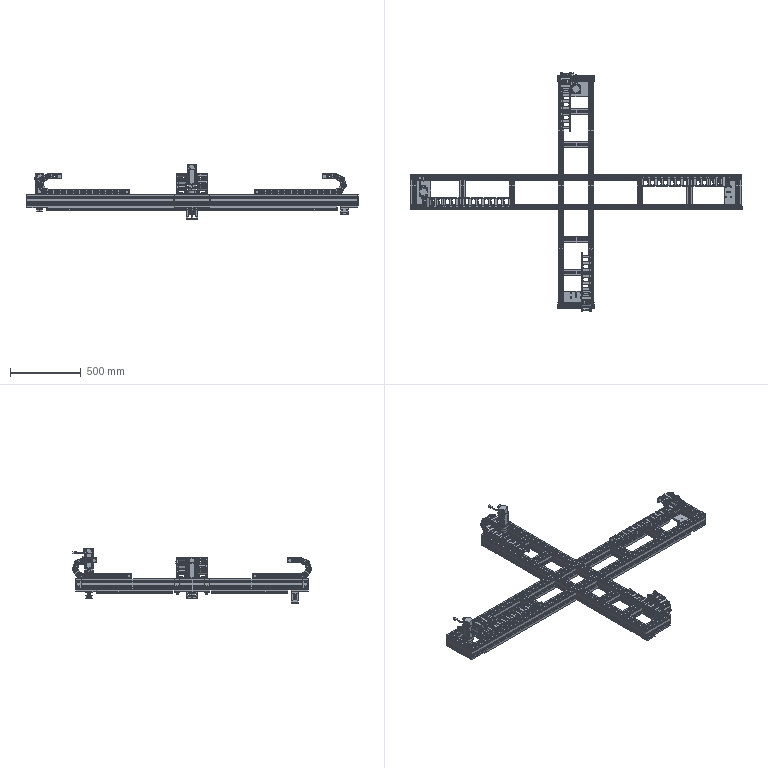Part | SolidWorks | features ReferencePattern 14, InContextFeatHolder 8, Belt 2, LocalCirPattern 2, MirrorCompFeat 1, RefAxis 1 | 153 solids | 25681 faces | volume 17712446 mm3 | plane 13130 | cylinder 11641 | cone 484 | spline 362 | torus 64 | commonest cylinder face diameters 2 x2378 4.24 x648 10 x521 18.2 x464 32.34 x448 13.7 x432